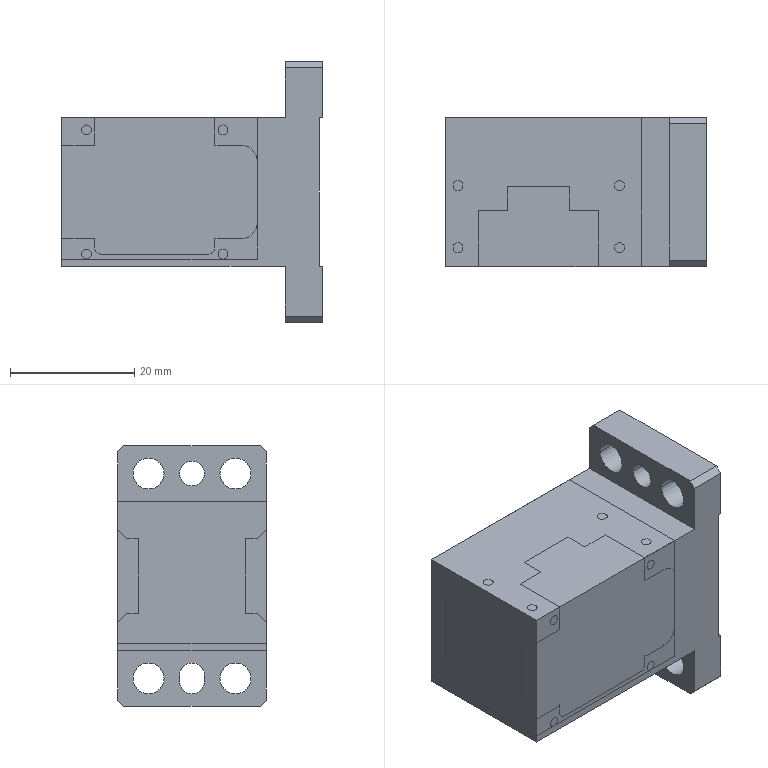NC program | NX | posted with a generic post | part box 42 x 24 x 42 mm
Whole program:
N10 G17 G21 G94 G90
(FLOOR_WALL_COPY , TOOL : D63)
N12 T01 M6
N14 G54
N16 G17 G0 G90 X55.5 Y0. B0. C0. S2000 M3
N18 G43 Z30. H1
N20 Z5.8
N22 G94 G1 Z2.8 F1000.
N24 X52.5
N26 X-52.5
N28 X-55.5
N30 Z5.8
N32 G0 Z30.
N34 X55.5
N36 Z5.6
N38 G1 Z2.6
N40 X52.5
N42 X-52.5
N44 X-55.5
N46 Z5.6
N48 G0 Z30.
N50 X55.5
N52 Z5.4
N54 G1 Z2.4
N56 X52.5
N58 X-52.5
N60 X-55.5
N62 Z5.4
N64 G0 Z30.
N66 X55.5
N68 Z5.2
N70 G1 Z2.2
N72 X52.5
N74 X-52.5
N76 X-55.5
N78 Z5.2
N80 G0 Z30.
N82 X55.5
N84 Z5.
N86 G1 Z2.
N88 X52.5
N90 X-52.5
N92 X-55.5
N94 Z5.
N96 G0 Z30.
N98 X55.5
N100 Z4.8
N102 G1 Z1.8
N104 X52.5
N106 X-52.5
N108 X-55.5
N110 Z4.8
N112 G0 Z30.
N114 X55.5
N116 Z4.6
N118 G1 Z1.6
N120 X52.5
N122 X-52.5
N124 X-55.5
N126 Z4.6
N128 G0 Z30.
N130 X55.5
N132 Z4.4
N134 G1 Z1.4
N136 X52.5
N138 X-52.5
N140 X-55.5
N142 Z4.4
N144 G0 Z30.
N146 X55.5
N148 Z4.2
N150 G1 Z1.2
N152 X52.5
N154 X-52.5
N156 X-55.5
N158 Z4.2
N160 G0 Z30.
N162 X55.5
N164 Z4.
N166 G1 Z1.
N168 X52.5
N170 X-52.5
N172 X-55.5
N174 Z4.
N176 G0 Z30.
N178 X55.5
N180 Z3.8
N182 G1 Z0.8
N184 X52.5
N186 X-52.5
N188 X-55.5
N190 Z3.8
N192 G0 Z30.
N194 X55.5
N196 Z3.6
N198 G1 Z0.6
N200 X52.5
N202 X-52.5
N204 X-55.5
N206 Z3.6
N208 G0 Z30.
N210 X55.5
N212 Z3.4
N214 G1 Z0.4
N216 X52.5
N218 X-52.5
N220 X-55.5
N222 Z3.4
N224 G0 Z30.
N226 X55.5
N228 Z3.2
N230 G1 Z0.2
N232 X52.5
N234 X-52.5
N236 X-55.5
N238 Z3.2
N240 G0 Z30.
N242 X55.5
N244 Z3.
N246 G1 Z0.
N248 X52.5
N250 X-52.5
N252 X-55.5
N254 Z3.
N256 G0 Z30.
N258 M5
(FLOOR_WALL_1_COPY , TOOL : D10)
N260 T10 M6
N262 G54
N264 G17 G0 G90 X1.22 Y18.5 B0. C0. S3000 M3
N266 G43 Z30. H10
N268 Z1.352
N270 G94 G1 Z-0.148 F1000.
N272 X4.684 Y12.5
N274 G3 X5.55 Y12. R1.
N276 G1 X16. F2000.
N278 X21.
N280 Y-12.
N282 X-9.9
N284 Y12.
N286 X5.55
N288 Y7.
N290 X16.
N292 Y-7.
N294 X-4.9
N296 Y7.
N298 X5.55
N300 Y2.
N302 X11.
N304 Y-2.
N306 X0.1
N308 Y2.
N310 X5.55
N312 G3 X6.416 Y2.5 R1.
N314 G1 Z1.352
N316 G0 X1.22 Y18.5 Z1.203
N318 G1 Z-0.297 F1000.
N320 X4.684 Y12.5
N322 G3 X5.55 Y12. R1.
N324 G1 X16. F2000.
N326 X21.
N328 Y-12.
N330 X-9.9
N332 Y12.
N334 X5.55
N336 Y7.
N338 X16.
N340 Y-7.
N342 X-4.9
N344 Y7.
N346 X5.55
N348 Y2.
N350 X11.
N352 Y-2.
N354 X0.1
N356 Y2.
N358 X5.55
N360 G3 X6.416 Y2.5 R1.
N362 G1 Z1.203
N364 G0 X1.22 Y18.5 Z1.055
N366 G1 Z-0.445 F1000.
N368 X4.684 Y12.5
N370 G3 X5.55 Y12. R1.
N372 G1 X16. F2000.
N374 X21.
N376 Y-12.
N378 X-9.9
N380 Y12.
N382 X5.55
N384 Y7.
N386 X16.
N388 Y-7.
N390 X-4.9
N392 Y7.
N394 X5.55
N396 Y2.
N398 X11.
N400 Y-2.
N402 X0.1
N404 Y2.
N406 X5.55
N408 G3 X6.416 Y2.5 R1.
N410 G1 Z1.055
N412 G0 X1.22 Y18.5 Z0.907
N414 G1 Z-0.593 F1000.
N416 X4.684 Y12.5
N418 G3 X5.55 Y12. R1.
N420 G1 X16. F2000.
N422 X21.
N424 Y-12.
N426 X-9.9
N428 Y12.
N430 X5.55
N432 Y7.
N434 X16.
N436 Y-7.
N438 X-4.9
N440 Y7.
N442 X5.55
N444 Y2.
N446 X11.
N448 Y-2.
N450 X0.1
N452 Y2.
N454 X5.55
N456 G3 X6.416 Y2.5 R1.
N458 G1 Z0.907
N460 G0 X1.22 Y18.5 Z0.758
N462 G1 Z-0.742 F1000.
N464 X4.684 Y12.5
N466 G3 X5.55 Y12. R1.
N468 G1 X16. F2000.
N470 X21.
N472 Y-12.
N474 X-9.9
N476 Y12.
N478 X5.55
N480 Y7.
N482 X16.
N484 Y-7.
N486 X-4.9
N488 Y7.
N490 X5.55
N492 Y2.
N494 X11.
N496 Y-2.
N498 X0.1
N500 Y2.
N502 X5.55
N504 G3 X6.416 Y2.5 R1.
N506 G1 Z0.758
N508 G0 X1.22 Y18.5 Z0.61
N510 G1 Z-0.89 F1000.
N512 X4.684 Y12.5
N514 G3 X5.55 Y12. R1.
N516 G1 X16. F2000.
N518 X21.
N520 Y-12.
N522 X-9.9
N524 Y12.
N526 X5.55
N528 Y7.
N530 X16.
N532 Y-7.
N534 X-4.9
N536 Y7.
N538 X5.55
N540 Y2.
N542 X11.
N544 Y-2.
N546 X0.1
N548 Y2.
N550 X5.55
N552 G3 X6.416 Y2.5 R1.
N554 G1 Z0.61
N556 G0 X1.22 Y18.5 Z0.462
N558 G1 Z-1.038 F1000.
N560 X4.684 Y12.5
N562 G3 X5.55 Y12. R1.
N564 G1 X16. F2000.
N566 X21.
N568 Y-12.
N570 X-9.9
N572 Y12.
N574 X5.55
N576 Y7.
N578 X16.
N580 Y-7.
N582 X-4.9
N584 Y7.
N586 X5.55
N588 Y2.
N590 X11.
N592 Y-2.
N594 X0.1
N596 Y2.
N598 X5.55
N600 G3 X6.416 Y2.5 R1.
N602 G1 Z0.462
N604 G0 X1.22 Y18.5 Z0.313
N606 G1 Z-1.187 F1000.
N608 X4.684 Y12.5
N610 G3 X5.55 Y12. R1.
N612 G1 X16. F2000.
N614 X21.
N616 Y-12.
N618 X-9.9
N620 Y12.
N622 X5.55
N624 Y7.
N626 X16.
N628 Y-7.
N630 X-4.9
N632 Y7.
N634 X5.55
N636 Y2.
N638 X11.
N640 Y-2.
N642 X0.1
N644 Y2.
N646 X5.55
N648 G3 X6.416 Y2.5 R1.
N650 G1 Z0.313
N652 G0 X1.22 Y18.5 Z0.165
N654 G1 Z-1.335 F1000.
N656 X4.684 Y12.5
N658 G3 X5.55 Y12. R1.
N660 G1 X16. F2000.
N662 X21.
N664 Y-12.
N666 X-9.9
N668 Y12.
N670 X5.55
N672 Y7.
N674 X16.
N676 Y-7.
N678 X-4.9
N680 Y7.
N682 X5.55
N684 Y2.
N686 X11.
N688 Y-2.
N690 X0.1
N692 Y2.
N694 X5.55
N696 G3 X6.416 Y2.5 R1.
N698 G1 Z0.165
N700 G0 X1.22 Y18.5 Z0.017
N702 G1 Z-1.483 F1000.
N704 X4.684 Y12.5
N706 G3 X5.55 Y12. R1.
N708 G1 X16. F2000.
N710 X21.
N712 Y-12.
N714 X-9.9
N716 Y12.
N718 X5.55
N720 Y7.
N722 X16.
N724 Y-7.
N726 X-4.9
N728 Y7.
N730 X5.55
N732 Y2.
N734 X11.
N736 Y-2.
N738 X0.1
N740 Y2.
N742 X5.55
N744 G3 X6.416 Y2.5 R1.
N746 G1 Z0.017
N748 G0 X1.22 Y18.5 Z-0.132
N750 G1 Z-1.632 F1000.
N752 X4.684 Y12.5
N754 G3 X5.55 Y12. R1.
N756 G1 X16. F2000.
N758 X21.
N760 Y-12.
N762 X-9.9
N764 Y12.
N766 X5.55
N768 Y7.
N770 X16.
N772 Y-7.
N774 X-4.9
N776 Y7.
N778 X5.55
N780 Y2.
N782 X11.
N784 Y-2.
N786 X0.1
N788 Y2.
N790 X5.55
N792 G3 X6.416 Y2.5 R1.
N794 G1 Z-0.132
N796 G0 X1.22 Y18.5 Z-0.28
N798 G1 Z-1.78 F1000.
N800 X4.684 Y12.5
N802 G3 X5.55 Y12. R1.
N804 G1 X16. F2000.
N806 X21.
N808 Y-12.
N810 X-9.9
N812 Y12.
N814 X5.55
N816 Y7.
N818 X16.
N820 Y-7.
N822 X-4.9
N824 Y7.
N826 X5.55
N828 Y2.
N830 X11.
N832 Y-2.
N834 X0.1
N836 Y2.
N838 X5.55
N840 G3 X6.416 Y2.5 R1.
N842 G1 Z-0.28
N844 G0 X1.22 Y18.5 Z-0.428
N846 G1 Z-1.928 F1000.
N848 X4.684 Y12.5
N850 G3 X5.55 Y12. R1.
N852 G1 X16. F2000.
N854 X21.
N856 Y-12.
N858 X-9.9
N860 Y12.
N862 X5.55
N864 Y7.
N866 X16.
N868 Y-7.
N870 X-4.9
N872 Y7.
N874 X5.55
N876 Y2.
N878 X11.
N880 Y-2.
N882 X0.1
N884 Y2.
N886 X5.55
N888 G3 X6.416 Y2.5 R1.
N890 G1 Z-0.428
N892 G0 X1.22 Y18.5 Z-0.577
N894 G1 Z-2.077 F1000.
N896 X4.684 Y12.5
N898 G3 X5.55 Y12. R1.
N900 G1 X16. F2000.
N902 X21.
N904 Y-12.
N906 X-9.9
N908 Y12.
N910 X5.55
N912 Y7.
N914 X16.
N916 Y-7.
N918 X-4.9
N920 Y7.
N922 X5.55
N924 Y2.
N926 X11.
N928 Y-2.
N930 X0.1
N932 Y2.
N934 X5.55
N936 G3 X6.416 Y2.5 R1.
N938 G1 Z-0.577
N940 G0 X1.22 Y18.5 Z-0.725
N942 G1 Z-2.225 F1000.
N944 X4.684 Y12.5
N946 G3 X5.55 Y12. R1.
N948 G1 X16. F2000.
N950 X21.
N952 Y-12.
N954 X-9.9
N956 Y12.
N958 X5.55
N960 Y7.
N962 X16.
N964 Y-7.
N966 X-4.9
N968 Y7.
N970 X5.55
N972 Y2.
N974 X11.
N976 Y-2.
N978 X0.1
N980 Y2.
N982 X5.55
N984 G3 X6.416 Y2.5 R1.
N986 G1 Z-0.725
N988 G0 X1.22 Y18.5 Z-0.873
N990 G1 Z-2.373 F1000.
N992 X4.684 Y12.5
N994 G3 X5.55 Y12. R1.
N996 G1 X16. F2000.
N998 X21.
N1000 Y-12.
N1002 X-9.9
N1004 Y12.
N1006 X5.55
N1008 Y7.
N1010 X16.
N1012 Y-7.
N1014 X-4.9
N1016 Y7.
N1018 X5.55
N1020 Y2.
N1022 X11.
N1024 Y-2.
N1026 X0.1
N1028 Y2.
N1030 X5.55
N1032 G3 X6.416 Y2.5 R1.
N1034 G1 Z-0.873
N1036 G0 X1.22 Y18.5 Z-1.022
N1038 G1 Z-2.522 F1000.
N1040 X4.684 Y12.5
N1042 G3 X5.55 Y12. R1.
N1044 G1 X16. F2000.
N1046 X21.
N1048 Y-12.
N1050 X-9.9
N1052 Y12.
N1054 X5.55
N1056 Y7.
N1058 X16.
N1060 Y-7.
N1062 X-4.9
N1064 Y7.
N1066 X5.55
N1068 Y2.
N1070 X11.
N1072 Y-2.
N1074 X0.1
N1076 Y2.
N1078 X5.55
N1080 G3 X6.416 Y2.5 R1.
N1082 G1 Z-1.022
N1084 G0 X1.22 Y18.5 Z-1.17
N1086 G1 Z-2.67 F1000.
N1088 X4.684 Y12.5
N1090 G3 X5.55 Y12. R1.
N1092 G1 X16. F2000.
N1094 X21.
N1096 Y-12.
N1098 X-9.9
N1100 Y12.
N1102 X5.55
N1104 Y7.
N1106 X16.
N1108 Y-7.
N1110 X-4.9
N1112 Y7.
N1114 X5.55
N1116 Y2.
N1118 X11.
N1120 Y-2.
N1122 X0.1
N1124 Y2.
N1126 X5.55
N1128 G3 X6.416 Y2.5 R1.
N1130 G1 Z-1.17
N1132 G0 X1.22 Y18.5 Z-1.318
N1134 G1 Z-2.818 F1000.
N1136 X4.684 Y12.5
N1138 G3 X5.55 Y12. R1.
N1140 G1 X16. F2000.
N1142 X21.
N1144 Y-12.
N1146 X-9.9
N1148 Y12.
N1150 X5.55
N1152 Y7.
N1154 X16.
N1156 Y-7.
N1158 X-4.9
N1160 Y7.
N1162 X5.55
N1164 Y2.
N1166 X11.
N1168 Y-2.
N1170 X0.1
N1172 Y2.
N1174 X5.55
N1176 G3 X6.416 Y2.5 R1.
N1178 G1 Z-1.318
N1180 G0 X1.22 Y18.5 Z-1.467
N1182 G1 Z-2.967 F1000.
N1184 X4.684 Y12.5
N1186 G3 X5.55 Y12. R1.
N1188 G1 X16. F2000.
N1190 X21.
N1192 Y-12.
N1194 X-9.9
N1196 Y12.
N1198 X5.55
N1200 Y7.
N1202 X16.
N1204 Y-7.
N1206 X-4.9
N1208 Y7.
N1210 X5.55
N1212 Y2.
N1214 X11.
N1216 Y-2.
N1218 X0.1
N1220 Y2.
N1222 X5.55
N1224 G3 X6.416 Y2.5 R1.
N1226 G1 Z-1.467
N1228 G0 X1.22 Y18.5 Z-1.615
N1230 G1 Z-3.115 F1000.
N1232 X4.684 Y12.5
N1234 G3 X5.55 Y12. R1.
N1236 G1 X16. F2000.
N1238 X21.
N1240 Y-12.
N1242 X-9.9
N1244 Y12.
N1246 X5.55
N1248 Y7.
N1250 X16.
N1252 Y-7.
N1254 X-4.9
N1256 Y7.
N1258 X5.55
N1260 Y2.
N1262 X11.
N1264 Y-2.
N1266 X0.1
N1268 Y2.
N1270 X5.55
N1272 G3 X6.416 Y2.5 R1.
N1274 G1 Z-1.615
N1276 G0 X1.22 Y18.5 Z-1.763
N1278 G1 Z-3.263 F1000.
N1280 X4.684 Y12.5
N1282 G3 X5.55 Y12. R1.
N1284 G1 X16. F2000.
N1286 X21.
N1288 Y-12.
N1290 X-9.9
N1292 Y12.
N1294 X5.55
N1296 Y7.
N1298 X16.
N1300 Y-7.
N1302 X-4.9
N1304 Y7.
N1306 X5.55
N1308 Y2.
N1310 X11.
N1312 Y-2.
N1314 X0.1
N1316 Y2.
N1318 X5.55
N1320 G3 X6.416 Y2.5 R1.
N1322 G1 Z-1.763
N1324 G0 X1.22 Y18.5 Z-1.912
N1326 G1 Z-3.412 F1000.
N1328 X4.684 Y12.5
N1330 G3 X5.55 Y12. R1.
N1332 G1 X16. F2000.
N1334 X21.
N1336 Y-12.
N1338 X-9.9
N1340 Y12.
N1342 X5.55
N1344 Y7.
N1346 X16.
N1348 Y-7.
N1350 X-4.9
N1352 Y7.
N1354 X5.55
N1356 Y2.
N1358 X11.
N1360 Y-2.
N1362 X0.1
N1364 Y2.
N1366 X5.55
N1368 G3 X6.416 Y2.5 R1.
N1370 G1 Z-1.912
N1372 G0 X1.22 Y18.5 Z-2.06
N1374 G1 Z-3.56 F1000.
N1376 X4.684 Y12.5
N1378 G3 X5.55 Y12. R1.
N1380 G1 X16. F2000.
N1382 X21.
N1384 Y-12.
N1386 X-9.9
N1388 Y12.
N1390 X5.55
N1392 Y7.
N1394 X16.
N1396 Y-7.
N1398 X-4.9
N1400 Y7.
N1402 X5.55
N1404 Y2.
N1406 X11.
N1408 Y-2.
N1410 X0.1
N1412 Y2.
N1414 X5.55
N1416 G3 X6.416 Y2.5 R1.
N1418 G1 Z-2.06
N1420 G0 X1.22 Y18.5 Z-2.208
N1422 G1 Z-3.708 F1000.
N1424 X4.684 Y12.5
N1426 G3 X5.55 Y12. R1.
N1428 G1 X16. F2000.
N1430 X21.
N1432 Y-12.
N1434 X-9.9
N1436 Y12.
N1438 X5.55
N1440 Y7.
N1442 X16.
N1444 Y-7.
N1446 X-4.9
N1448 Y7.
N1450 X5.55
N1452 Y2.
N1454 X11.
N1456 Y-2.
N1458 X0.1
N1460 Y2.
N1462 X5.55
N1464 G3 X6.416 Y2.5 R1.
N1466 G1 Z-2.208
N1468 G0 X1.22 Y18.5 Z-2.357
N1470 G1 Z-3.857 F1000.
N1472 X4.684 Y12.5
N1474 G3 X5.55 Y12. R1.
N1476 G1 X16. F2000.
N1478 X21.
N1480 Y-12.
N1482 X-9.9
N1484 Y12.
N1486 X5.55
N1488 Y7.
N1490 X16.
N1492 Y-7.
N1494 X-4.9
N1496 Y7.
N1498 X5.55
N1500 Y2.
N1502 X11.
N1504 Y-2.
N1506 X0.1
N1508 Y2.
N1510 X5.55
N1512 G3 X6.416 Y2.5 R1.
N1514 G1 Z-2.357
N1516 G0 X1.22 Y18.5 Z-2.505
N1518 G1 Z-4.005 F1000.
N1520 X4.684 Y12.5
N1522 G3 X5.55 Y12. R1.
N1524 G1 X16. F2000.
N1526 X21.
N1528 Y-12.
N1530 X-9.9
N1532 Y12.
N1534 X5.55
N1536 Y7.
N1538 X16.
N1540 Y-7.
N1542 X-4.9
N1544 Y7.
N1546 X5.55
N1548 Y2.
N1550 X11.
N1552 Y-2.
N1554 X0.1
N1556 Y2.
N1558 X5.55
N1560 G3 X6.416 Y2.5 R1.
N1562 G1 Z-2.505
N1564 G0 X1.22 Y18.5 Z-2.653
N1566 G1 Z-4.153 F1000.
N1568 X4.684 Y12.5
N1570 G3 X5.55 Y12. R1.
N1572 G1 X16. F2000.
N1574 X21.
N1576 Y-12.
N1578 X-9.9
N1580 Y12.
N1582 X5.55
N1584 Y7.
N1586 X16.
N1588 Y-7.
N1590 X-4.9
N1592 Y7.
N1594 X5.55
N1596 Y2.
N1598 X11.
N1600 Y-2.
N1602 X0.1
N1604 Y2.
N1606 X5.55
N1608 G3 X6.416 Y2.5 R1.
N1610 G1 Z-2.653
N1612 G0 X1.22 Y18.5 Z-2.802
N1614 G1 Z-4.302 F1000.
N1616 X4.684 Y12.5
N1618 G3 X5.55 Y12. R1.
N1620 G1 X16. F2000.
N1622 X21.
N1624 Y-12.
N1626 X-9.9
N1628 Y12.
N1630 X5.55
N1632 Y7.
N1634 X16.
N1636 Y-7.
N1638 X-4.9
N1640 Y7.
N1642 X5.55
N1644 Y2.
N1646 X11.
N1648 Y-2.
N1650 X0.1
N1652 Y2.
N1654 X5.55
N1656 G3 X6.416 Y2.5 R1.
N1658 G1 Z-2.802
N1660 G0 X1.22 Y18.5 Z-2.95
N1662 G1 Z-4.45 F1000.
N1664 X4.684 Y12.5
N1666 G3 X5.55 Y12. R1.
N1668 G1 X16. F2000.
N1670 X21.
N1672 Y-12.
N1674 X-9.9
N1676 Y12.
N1678 X5.55
N1680 Y7.
N1682 X16.
N1684 Y-7.
N1686 X-4.9
N1688 Y7.
N1690 X5.55
N1692 Y2.
N1694 X11.
N1696 Y-2.
N1698 X0.1
N1700 Y2.
N1702 X5.55
N1704 G3 X6.416 Y2.5 R1.
N1706 G1 Z-2.95
N1708 G0 X1.22 Y18.5 Z-3.098
N1710 G1 Z-4.598 F1000.
N1712 X4.684 Y12.5
N1714 G3 X5.55 Y12. R1.
N1716 G1 X16. F2000.
N1718 X21.
N1720 Y-12.
N1722 X-9.9
N1724 Y12.
N1726 X5.55
N1728 Y7.
N1730 X16.
N1732 Y-7.
N1734 X-4.9
N1736 Y7.
N1738 X5.55
N1740 Y2.
N1742 X11.
N1744 Y-2.
N1746 X0.1
N1748 Y2.
N1750 X5.55
N1752 G3 X6.416 Y2.5 R1.
N1754 G1 Z-3.098
N1756 G0 X1.22 Y18.5 Z-3.247
N1758 G1 Z-4.747 F1000.
N1760 X4.684 Y12.5
N1762 G3 X5.55 Y12. R1.
N1764 G1 X16. F2000.
N1766 X21.
N1768 Y-12.
N1770 X-9.9
N1772 Y12.
N1774 X5.55
N1776 Y7.
N1778 X16.
N1780 Y-7.
N1782 X-4.9
N1784 Y7.
N1786 X5.55
N1788 Y2.
N1790 X11.
N1792 Y-2.
N1794 X0.1
N1796 Y2.
N1798 X5.55
N1800 G3 X6.416 Y2.5 R1.
N1802 G1 Z-3.247
N1804 G0 X1.22 Y18.5 Z-3.395
N1806 G1 Z-4.895 F1000.
N1808 X4.684 Y12.5
N1810 G3 X5.55 Y12. R1.
N1812 G1 X16. F2000.
N1814 X21.
N1816 Y-12.
N1818 X-9.9
N1820 Y12.
N1822 X5.55
N1824 Y7.
N1826 X16.
N1828 Y-7.
N1830 X-4.9
N1832 Y7.
N1834 X5.55
N1836 Y2.
N1838 X11.
N1840 Y-2.
N1842 X0.1
N1844 Y2.
N1846 X5.55
N1848 G3 X6.416 Y2.5 R1.
N1850 G1 Z-3.395
N1852 G0 X1.22 Y18.5 Z-3.543
N1854 G1 Z-5.043 F1000.
N1856 X4.684 Y12.5
N1858 G3 X5.55 Y12. R1.
N1860 G1 X16. F2000.
N1862 X21.
N1864 Y-12.
N1866 X-9.9
N1868 Y12.
N1870 X5.55
N1872 Y7.
N1874 X16.
N1876 Y-7.
N1878 X-4.9
N1880 Y7.
N1882 X5.55
N1884 Y2.
N1886 X11.
N1888 Y-2.
N1890 X0.1
N1892 Y2.
N1894 X5.55
N1896 G3 X6.416 Y2.5 R1.
N1898 G1 Z-3.543
N1900 G0 X1.22 Y18.5 Z-3.692
N1902 G1 Z-5.192 F1000.
N1904 X4.684 Y12.5
N1906 G3 X5.55 Y12. R1.
N1908 G1 X16. F2000.
N1910 X21.
N1912 Y-12.
N1914 X-9.9
N1916 Y12.
N1918 X5.55
N1920 Y7.
N1922 X16.
N1924 Y-7.
N1926 X-4.9
N1928 Y7.
N1930 X5.55
N1932 Y2.
N1934 X11.
N1936 Y-2.
N1938 X0.1
N1940 Y2.
N1942 X5.55
N1944 G3 X6.416 Y2.5 R1.
N1946 G1 Z-3.692
N1948 G0 X1.22 Y18.5 Z-3.84
N1950 G1 Z-5.34 F1000.
N1952 X4.684 Y12.5
N1954 G3 X5.55 Y12. R1.
N1956 G1 X16. F2000.
N1958 X21.
N1960 Y-12.
N1962 X-9.9
N1964 Y12.
N1966 X5.55
N1968 Y7.
N1970 X16.
N1972 Y-7.
N1974 X-4.9
N1976 Y7.
N1978 X5.55
N1980 Y2.
N1982 X11.
N1984 Y-2.
N1986 X0.1
N1988 Y2.
N1990 X5.55
N1992 G3 X6.416 Y2.5 R1.
N1994 G1 Z-3.84
N1996 G0 X1.22 Y18.5 Z-3.988
N1998 G1 Z-5.488 F1000.
N2000 X4.684 Y12.5
N2002 G3 X5.55 Y12. R1.
N2004 G1 X16. F2000.
N2006 X21.
N2008 Y-12.
N2010 X-9.9
N2012 Y12.
N2014 X5.55
N2016 Y7.
N2018 X16.
N2020 Y-7.
N2022 X-4.9
N2024 Y7.
N2026 X5.55
N2028 Y2.
N2030 X11.
N2032 Y-2.
N2034 X0.1
N2036 Y2.
N2038 X5.55
N2040 G3 X6.416 Y2.5 R1.
N2042 G1 Z-3.988
N2044 G0 X1.22 Y18.5 Z-4.137
N2046 G1 Z-5.637 F1000.
N2048 X4.684 Y12.5
N2050 G3 X5.55 Y12. R1.
N2052 G1 X16. F2000.
N2054 X21.
N2056 Y-12.
N2058 X-9.9
N2060 Y12.
N2062 X5.55
N2064 Y7.
N2066 X16.
N2068 Y-7.
N2070 X-4.9
N2072 Y7.
N2074 X5.55
N2076 Y2.
N2078 X11.
N2080 Y-2.
N2082 X0.1
N2084 Y2.
N2086 X5.55
N2088 G3 X6.416 Y2.5 R1.
N2090 G1 Z-4.137
N2092 G0 X1.22 Y18.5 Z-4.285
N2094 G1 Z-5.785 F1000.
N2096 X4.684 Y12.5
N2098 G3 X5.55 Y12. R1.
N2100 G1 X16. F2000.
N2102 X21.
N2104 Y-12.
N2106 X-9.9
N2108 Y12.
N2110 X5.55
N2112 Y7.
N2114 X16.
N2116 Y-7.
N2118 X-4.9
N2120 Y7.
N2122 X5.55
N2124 Y2.
N2126 X11.
N2128 Y-2.
N2130 X0.1
N2132 Y2.
N2134 X5.55
N2136 G3 X6.416 Y2.5 R1.
N2138 G1 Z-4.285
N2140 G0 X1.22 Y18.5 Z-4.433
N2142 G1 Z-5.933 F1000.
N2144 X4.684 Y12.5
N2146 G3 X5.55 Y12. R1.
N2148 G1 X16. F2000.
N2150 X21.
N2152 Y-12.
N2154 X-9.9
N2156 Y12.
N2158 X5.55
N2160 Y7.
N2162 X16.
N2164 Y-7.
N2166 X-4.9
N2168 Y7.
N2170 X5.55
N2172 Y2.
N2174 X11.
N2176 Y-2.
N2178 X0.1
N2180 Y2.
N2182 X5.55
N2184 G3 X6.416 Y2.5 R1.
N2186 G1 Z-4.433
N2188 G0 X1.22 Y18.5 Z-4.582
N2190 G1 Z-6.082 F1000.
N2192 X4.684 Y12.5
N2194 G3 X5.55 Y12. R1.
N2196 G1 X16. F2000.
N2198 X21.
N2200 Y-12.
N2202 X-9.9
N2204 Y12.
N2206 X5.55
N2208 Y7.
N2210 X16.
N2212 Y-7.
N2214 X-4.9
N2216 Y7.
N2218 X5.55
N2220 Y2.
N2222 X11.
N2224 Y-2.
N2226 X0.1
N2228 Y2.
N2230 X5.55
N2232 G3 X6.416 Y2.5 R1.
N2234 G1 Z-4.582
N2236 G0 X1.22 Y18.5 Z-4.73
N2238 G1 Z-6.23 F1000.
N2240 X4.684 Y12.5
N2242 G3 X5.55 Y12. R1.
N2244 G1 X16. F2000.
N2246 X21.
N2248 Y-12.
N2250 X-9.9
N2252 Y12.
N2254 X5.55
N2256 Y7.
N2258 X16.
N2260 Y-7.
N2262 X-4.9
N2264 Y7.
N2266 X5.55
N2268 Y2.
N2270 X11.
N2272 Y-2.
N2274 X0.1
N2276 Y2.
N2278 X5.55
N2280 G3 X6.416 Y2.5 R1.
N2282 G1 Z-4.73
N2284 G0 X1.22 Y18.5 Z-4.878
N2286 G1 Z-6.378 F1000.
N2288 X4.684 Y12.5
N2290 G3 X5.55 Y12. R1.
N2292 G1 X16. F2000.
N2294 X21.
N2296 Y-12.
N2298 X-9.9
N2300 Y12.
N2302 X5.55
N2304 Y7.
N2306 X16.
N2308 Y-7.
N2310 X-4.9
N2312 Y7.
N2314 X5.55
N2316 Y2.
N2318 X11.
N2320 Y-2.
N2322 X0.1
N2324 Y2.
N2326 X5.55
N2328 G3 X6.416 Y2.5 R1.
N2330 G1 Z-4.878
N2332 G0 X1.22 Y18.5 Z-5.027
N2334 G1 Z-6.527 F1000.
N2336 X4.684 Y12.5
N2338 G3 X5.55 Y12. R1.
N2340 G1 X16. F2000.
N2342 X21.
N2344 Y-12.
N2346 X-9.9
N2348 Y12.
N2350 X5.55
N2352 Y7.
N2354 X16.
N2356 Y-7.
N2358 X-4.9
N2360 Y7.
N2362 X5.55
N2364 Y2.
N2366 X11.
N2368 Y-2.
N2370 X0.1
N2372 Y2.
N2374 X5.55
N2376 G3 X6.416 Y2.5 R1.
N2378 G1 Z-5.027
N2380 G0 X1.22 Y18.5 Z-5.175
N2382 G1 Z-6.675 F1000.
N2384 X4.684 Y12.5
N2386 G3 X5.55 Y12. R1.
N2388 G1 X16. F2000.
N2390 X21.
N2392 Y-12.
N2394 X-9.9
N2396 Y12.
N2398 X5.55
N2400 Y7.
N2402 X16.
N2404 Y-7.
N2406 X-4.9
N2408 Y7.
N2410 X5.55
N2412 Y2.
N2414 X11.
N2416 Y-2.
N2418 X0.1
N2420 Y2.
N2422 X5.55
N2424 G3 X6.416 Y2.5 R1.
N2426 G1 Z-5.175
N2428 G0 X1.22 Y18.5 Z-5.323
N2430 G1 Z-6.823 F1000.
N2432 X4.684 Y12.5
N2434 G3 X5.55 Y12. R1.
N2436 G1 X16. F2000.
N2438 X21.
N2440 Y-12.
N2442 X-9.9
N2444 Y12.
N2446 X5.55
N2448 Y7.
N2450 X16.
N2452 Y-7.
N2454 X-4.9
N2456 Y7.
N2458 X5.55
N2460 Y2.
N2462 X11.
N2464 Y-2.
N2466 X0.1
N2468 Y2.
N2470 X5.55
N2472 G3 X6.416 Y2.5 R1.
N2474 G1 Z-5.323
N2476 G0 X1.22 Y18.5 Z-5.472
N2478 G1 Z-6.972 F1000.
N2480 X4.684 Y12.5
N2482 G3 X5.55 Y12. R1.
N2484 G1 X16. F2000.
N2486 X21.
N2488 Y-12.
N2490 X-9.9
N2492 Y12.
N2494 X5.55
N2496 Y7.
N2498 X16.
N2500 Y-7.
N2502 X-4.9
N2504 Y7.
N2506 X5.55
N2508 Y2.
N2510 X11.
N2512 Y-2.
N2514 X0.1
N2516 Y2.
N2518 X5.55
N2520 G3 X6.416 Y2.5 R1.
N2522 G1 Z-5.472
N2524 G0 X1.22 Y18.5 Z-5.62
N2526 G1 Z-7.12 F1000.
N2528 X4.684 Y12.5
N2530 G3 X5.55 Y12. R1.
N2532 G1 X16. F2000.
N2534 X21.
N2536 Y-12.
N2538 X-9.9
N2540 Y12.
N2542 X5.55
N2544 Y7.
N2546 X16.
N2548 Y-7.
N2550 X-4.9
N2552 Y7.
N2554 X5.55
N2556 Y2.
N2558 X11.
N2560 Y-2.
N2562 X0.1
N2564 Y2.
N2566 X5.55
N2568 G3 X6.416 Y2.5 R1.
N2570 G1 Z-5.62
N2572 G0 X1.22 Y18.5 Z-5.768
N2574 G1 Z-7.268 F1000.
N2576 X4.684 Y12.5
N2578 G3 X5.55 Y12. R1.
N2580 G1 X16. F2000.
N2582 X21.
N2584 Y-12.
N2586 X-9.9
N2588 Y12.
N2590 X5.55
N2592 Y7.
N2594 X16.
N2596 Y-7.
N2598 X-4.9
N2600 Y7.
N2602 X5.55
N2604 Y2.
N2606 X11.
N2608 Y-2.
N2610 X0.1
N2612 Y2.
N2614 X5.55
N2616 G3 X6.416 Y2.5 R1.
N2618 G1 Z-5.768
N2620 G0 X1.22 Y18.5 Z-5.917
N2622 G1 Z-7.417 F1000.
N2624 X4.684 Y12.5
N2626 G3 X5.55 Y12. R1.
N2628 G1 X16. F2000.
N2630 X21.
N2632 Y-12.
N2634 X-9.9
N2636 Y12.
N2638 X5.55
N2640 Y7.
N2642 X16.
N2644 Y-7.
N2646 X-4.9
N2648 Y7.
N2650 X5.55
N2652 Y2.
N2654 X11.
N2656 Y-2.
N2658 X0.1
N2660 Y2.
N2662 X5.55
N2664 G3 X6.416 Y2.5 R1.
N2666 G1 Z-5.917
N2668 G0 X1.22 Y18.5 Z-6.065
N2670 G1 Z-7.565 F1000.
N2672 X4.684 Y12.5
N2674 G3 X5.55 Y12. R1.
N2676 G1 X16. F2000.
N2678 X21.
N2680 Y-12.
N2682 X-9.9
N2684 Y12.
N2686 X5.55
N2688 Y7.
N2690 X16.
N2692 Y-7.
N2694 X-4.9
N2696 Y7.
N2698 X5.55
N2700 Y2.
N2702 X11.
N2704 Y-2.
N2706 X0.1
N2708 Y2.
N2710 X5.55
N2712 G3 X6.416 Y2.5 R1.
N2714 G1 Z-6.065
N2716 G0 X1.22 Y18.5 Z-6.213
N2718 G1 Z-7.713 F1000.
N2720 X4.684 Y12.5
N2722 G3 X5.55 Y12. R1.
N2724 G1 X16. F2000.
N2726 X21.
N2728 Y-12.
N2730 X-9.9
N2732 Y12.
N2734 X5.55
N2736 Y7.
N2738 X16.
N2740 Y-7.
N2742 X-4.9
N2744 Y7.
N2746 X5.55
N2748 Y2.
N2750 X11.
N2752 Y-2.
N2754 X0.1
N2756 Y2.
N2758 X5.55
N2760 G3 X6.416 Y2.5 R1.
N2762 G1 Z-6.213
N2764 G0 X1.22 Y18.5 Z-6.362
N2766 G1 Z-7.862 F1000.
N2768 X4.684 Y12.5
N2770 G3 X5.55 Y12. R1.
N2772 G1 X16. F2000.
N2774 X21.
N2776 Y-12.
N2778 X-9.9
N2780 Y12.
N2782 X5.55
N2784 Y7.
N2786 X16.
N2788 Y-7.
N2790 X-4.9
N2792 Y7.
N2794 X5.55
N2796 Y2.
N2798 X11.
N2800 Y-2.
N2802 X0.1
N2804 Y2.
N2806 X5.55
N2808 G3 X6.416 Y2.5 R1.
N2810 G1 Z-6.362
N2812 G0 X1.22 Y18.5 Z-6.51
N2814 G1 Z-8.01 F1000.
N2816 X4.684 Y12.5
N2818 G3 X5.55 Y12. R1.
N2820 G1 X16. F2000.
N2822 X21.
N2824 Y-12.
N2826 X-9.9
N2828 Y12.
N2830 X5.55
N2832 Y7.
N2834 X16.
N2836 Y-7.
N2838 X-4.9
N2840 Y7.
N2842 X5.55
N2844 Y2.
N2846 X11.
N2848 Y-2.
N2850 X0.1
N2852 Y2.
N2854 X5.55
N2856 G3 X6.416 Y2.5 R1.
N2858 G1 Z-6.51
N2860 G0 X1.22 Y18.5 Z-6.658
N2862 G1 Z-8.158 F1000.
N2864 X4.684 Y12.5
N2866 G3 X5.55 Y12. R1.
N2868 G1 X16. F2000.
N2870 X21.
N2872 Y-12.
N2874 X-9.9
N2876 Y12.
N2878 X5.55
N2880 Y7.
N2882 X16.
N2884 Y-7.
N2886 X-4.9
N2888 Y7.
N2890 X5.55
N2892 Y2.
N2894 X11.
N2896 Y-2.
N2898 X0.1
N2900 Y2.
N2902 X5.55
N2904 G3 X6.416 Y2.5 R1.
N2906 G1 Z-6.658
N2908 G0 X1.22 Y18.5 Z-6.807
N2910 G1 Z-8.307 F1000.
N2912 X4.684 Y12.5
N2914 G3 X5.55 Y12. R1.
N2916 G1 X16. F2000.
N2918 X21.
N2920 Y-12.
N2922 X-9.9
N2924 Y12.
N2926 X5.55
N2928 Y7.
N2930 X16.
N2932 Y-7.
N2934 X-4.9
N2936 Y7.
N2938 X5.55
N2940 Y2.
N2942 X11.
N2944 Y-2.
N2946 X0.1
N2948 Y2.
N2950 X5.55
N2952 G3 X6.416 Y2.5 R1.
N2954 G1 Z-6.807
N2956 G0 X1.22 Y18.5 Z-6.955
N2958 G1 Z-8.455 F1000.
N2960 X4.684 Y12.5
N2962 G3 X5.55 Y12. R1.
N2964 G1 X16. F2000.
N2966 X21.
N2968 Y-12.
N2970 X-9.9
N2972 Y12.
N2974 X5.55
N2976 Y7.
N2978 X16.
N2980 Y-7.
N2982 X-4.9
N2984 Y7.
N2986 X5.55
N2988 Y2.
N2990 X11.
N2992 Y-2.
N2994 X0.1
N2996 Y2.
N2998 X5.55
N3000 G3 X6.416 Y2.5 R1.
N3002 G1 Z-6.955
N3004 G0 X1.22 Y18.5 Z-7.103
N3006 G1 Z-8.603 F1000.
N3008 X4.684 Y12.5
N3010 G3 X5.55 Y12. R1.
N3012 G1 X16. F2000.
N3014 X21.
N3016 Y-12.
N3018 X-9.9
N3020 Y12.
N3022 X5.55
N3024 Y7.
N3026 X16.
N3028 Y-7.
N3030 X-4.9
N3032 Y7.
N3034 X5.55
N3036 Y2.
N3038 X11.
N3040 Y-2.
N3042 X0.1
N3044 Y2.
N3046 X5.55
N3048 G3 X6.416 Y2.5 R1.
N3050 G1 Z-7.103
N3052 G0 X1.22 Y18.5 Z-7.252
N3054 G1 Z-8.752 F1000.
N3056 X4.684 Y12.5
N3058 G3 X5.55 Y12. R1.
N3060 G1 X16. F2000.
N3062 X21.
N3064 Y-12.
N3066 X-9.9
N3068 Y12.
N3070 X5.55
N3072 Y7.
N3074 X16.
N3076 Y-7.
N3078 X-4.9
N3080 Y7.
N3082 X5.55
N3084 Y2.
N3086 X11.
N3088 Y-2.
N3090 X0.1
N3092 Y2.
N3094 X5.55
N3096 G3 X6.416 Y2.5 R1.
N3098 G1 Z-7.252
N3100 G0 X1.22 Y18.5 Z-7.4
N3102 G1 Z-8.9 F1000.
N3104 X4.684 Y12.5
N3106 G3 X5.55 Y12. R1.
N3108 G1 X16. F2000.
N3110 X21.
N3112 Y-12.
N3114 X-9.9
N3116 Y12.
N3118 X5.55
N3120 Y7.
N3122 X16.
N3124 Y-7.
N3126 X-4.9
N3128 Y7.
N3130 X5.55
N3132 Y2.
N3134 X11.
N3136 Y-2.
N3138 X0.1
N3140 Y2.
N3142 X5.55
N3144 G3 X6.416 Y2.5 R1.
N3146 G1 Z-7.4
N3148 G0 Z30.
N3150 M5
(FLOOR_WALL_1_1_COPY , TOOL : D10JING)
N3152 T11 M6
N3154 G54
N3156 G17 G0 G90 X23.463 Y19. B0. C0. S5500 M3
N3158 G43 Z30. H11
N3160 Z-7.5
N3162 G94 G1 Z-9. F1250.
N3164 X21.499 Y17.866
N3166 G3 X20.999 Y17. R1.
N3168 G1 Y-17.
N3170 X16.642
N3172 Y17.
N3174 X12.285
N3176 Y-17.
N3178 X7.928
N3180 Y17.
N3182 X3.571
N3184 Y-17.
N3186 X-0.786
N3188 Y17.
N3190 X-5.143
N3192 Y-17.
N3194 X-9.5
N3196 Y17.
N3198 G2 X-9. Y17.866 R1.
N3200 G1 X-7.036 Y19.
N3202 Z-7.5
N3204 G0 Z30.
N3206 X-7.536
N3208 Z-7.5
N3210 G1 Z-9.
N3212 X-9.5 Y17.866
N3214 G3 X-10. Y17. R1.
N3216 G1 Y-17.
N3218 G3 X-9.5 Y-17.866 R1.
N3220 G1 X-7.536 Y-19.
N3222 Z-7.5
N3224 G0 Z30.
N3226 M5
(DRILLING , TOOL : D6A45)
N3228 T07 M6
N3230 G54
N3232 G17 G0 G90 X-7. Y-1. B0. C0. S5000 M3
N3234 G43 Z30. H7
N3236 G94 G81 G98 Z-10.1 F250. R-6.
N3238 X19.
N3240 X-7. Y9.
N3242 X19.
N3244 G80
N3246 G0 X19. Y9. Z30.
N3248 M5
(DRILLING_COPY , TOOL : 1.6ZT)
N3250 T16 M6
N3252 G54
N3254 G17 G0 G90 X-7. Y-1. B0. C0. S2000 M3
N3256 G43 Z30. H16
N3258 G94 G83 G98 Z-14.481 F100. Q2. R-6.
N3260 X19.
N3262 X-7. Y9.
N3264 X19.
N3266 G80
N3268 G0 X19. Y9. Z30.
N3270 M5
(PLANAR_MILL_COPY_1 , TOOL : D6A45)
N3272 T07 M6
N3274 G54
N3276 G17 G0 G90 X-10.908 Y14.313 B0. C0. S7500 M3
N3278 G43 Z30. H7
N3280 Z-8.5
N3282 G94 G1 Z-10. F1250.
N3284 X-11.357 Y13.865
N3286 G3 X-11.618 Y12.9 R1.
N3288 G1 X20.9
N3290 G2 X21.9 Y11.9 R1.
N3292 G1 Y-11.9
N3294 G2 X20.9 Y-12.9 R1.
N3296 G1 X-11.618
N3298 G3 X-11.357 Y-13.865 R1.
N3300 G1 X-10.908 Y-14.313
N3302 Z-8.5
N3304 G0 Z30.
(PLANAR_MILL_COPY_COPY , TOOL : D6A45)
N3306 X-11.9 Y1.27
N3308 Z-0.5
N3310 G1 Z-2.
N3312 X-12.6 Y0.866
N3314 G3 X-13.1 Y0. R1.
N3316 G1 Y-10.9
N3318 G2 X-15.1 Y-12.9 R2.
N3320 G1 X-20.9
N3322 G2 X-22.9 Y-10.9 R2.
N3324 G1 Y10.9
N3326 G2 X-20.9 Y12.9 R2.
N3328 G1 X-15.1
N3330 G2 X-13.1 Y10.9 R2.
N3332 G1 Y0.
N3334 G3 X-12.6 Y-0.866 R1.
N3336 G1 X-11.9 Y-1.27
N3338 Z-0.5
N3340 G0 Z30.
N3342 M5
N3344 M2